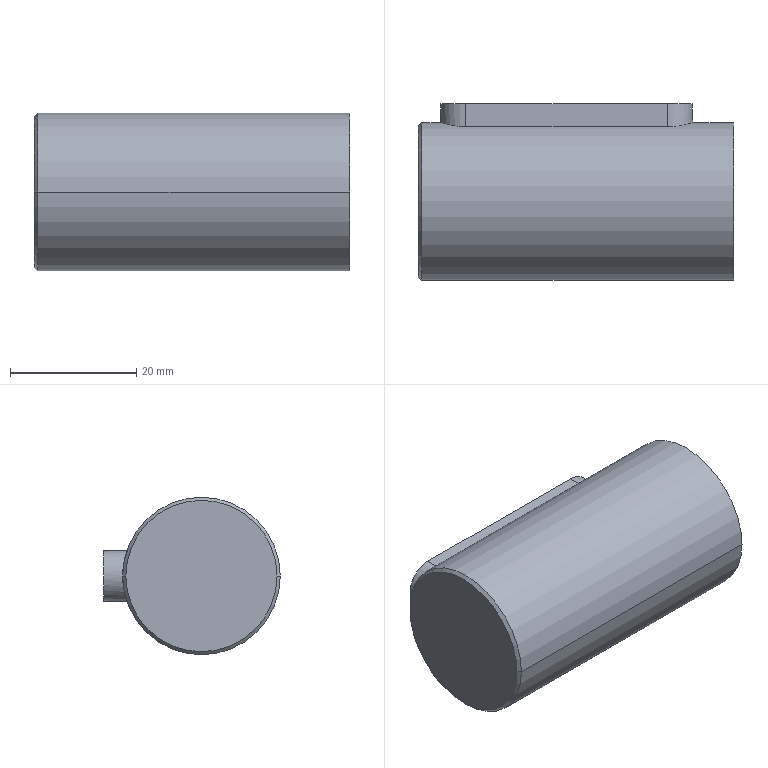Part | STEP file | PRODUCT_ID_83 | 1 solid | 11 faces | box 50 x 28 x 25 mm | volume 25516 mm3 | plane 5 | cylinder 4 | cone 2 | commonest cylinder face diameters 8 x2 25 x2
STEP:
#1=CARTESIAN_POINT('',(0.,0.,0.));
#2=DIRECTION('',(0.,0.,1.));
#3=DIRECTION('',(1.,0.,0.));
#4=AXIS2_PLACEMENT_3D('',#1,#2,#3);
#5=CARTESIAN_POINT('',(-42.5,15.5,4.));
#6=VERTEX_POINT('',#5);
#7=CARTESIAN_POINT('',(-42.5,15.5,-4.));
#8=VERTEX_POINT('',#7);
#9=CARTESIAN_POINT('',(-42.5,15.5,0.));
#10=DIRECTION('',(0.,-1.,0.));
#11=DIRECTION('',(0.,0.,1.));
#12=AXIS2_PLACEMENT_3D('',#9,#10,#11);
#13=CIRCLE('',#12,4.);
#14=CARTESIAN_POINT('',(-42.5,15.5,0.));
#15=DIRECTION('',(0.,1.,0.));
#16=DIRECTION('',(0.,0.,-1.));
#17=AXIS2_PLACEMENT_3D('',#14,#15,#16);
#18=PLANE('',#17);
#19=CARTESIAN_POINT('',(-4.,0.));
#20=CARTESIAN_POINT('',(-4.,6.928));
#21=CARTESIAN_POINT('',(2.,3.464));
#22=CARTESIAN_POINT('',(8.,0.));
#23=CARTESIAN_POINT('',(2.,-3.464));
#24=CARTESIAN_POINT('',(-4.,-6.928));
#25=CARTESIAN_POINT('',(-4.,0.));
#26=(BOUNDED_CURVE()B_SPLINE_CURVE(2,(#19,#20,#21,#22,#23,#24,#25),.UNSPECIFIED.,.T.,.F.)B_SPLINE_CURVE_WITH_KNOTS((1,2,2,2,2,1),(-2.094,0.,2.094,4.189,6.283,8.378),.UNSPECIFIED.)CURVE()GEOMETRIC_REPRESENTATION_ITEM()RATIONAL_B_SPLINE_CURVE((1.,0.5,1.,0.5,1.,0.5,1.))REPRESENTATION_ITEM(''));
#27=(GEOMETRIC_REPRESENTATION_CONTEXT(2)PARAMETRIC_REPRESENTATION_CONTEXT()REPRESENTATION_CONTEXT('',''));
#28=DEFINITIONAL_REPRESENTATION('',(#26),#27);
#29=PCURVE('',#18,#28);
#30=CARTESIAN_POINT('',(-42.5,7.75,0.));
#31=DIRECTION('',(0.,1.,0.));
#32=DIRECTION('',(0.,0.,1.));
#33=AXIS2_PLACEMENT_3D('',#30,#31,#32);
#34=CYLINDRICAL_SURFACE('',#33,4.);
#35=CARTESIAN_POINT('',(6.283,7.75));
#36=DIRECTION('',(-1.,0.));
#37=VECTOR('',#36,1.);
#38=LINE('',#35,#37);
#39=(GEOMETRIC_REPRESENTATION_CONTEXT(2)PARAMETRIC_REPRESENTATION_CONTEXT()REPRESENTATION_CONTEXT('',''));
#40=DEFINITIONAL_REPRESENTATION('',(#38),#39);
#41=PCURVE('',#34,#40);
#42=SURFACE_CURVE('',#13,(#29,#41),.PCURVE_S1.);
#43=EDGE_CURVE('',#6,#8,#42,.T.);
#44=ORIENTED_EDGE('',*,*,#43,.F.);
#45=CARTESIAN_POINT('',(-10.5,15.5,4.));
#46=VERTEX_POINT('',#45);
#47=CARTESIAN_POINT('',(-26.5,15.5,4.));
#48=DIRECTION('',(1.,0.,0.));
#49=VECTOR('',#48,1.);
#50=LINE('',#47,#49);
#51=CARTESIAN_POINT('',(-4.,-16.));
#52=DIRECTION('',(0.,-1.));
#53=VECTOR('',#52,1.);
#54=LINE('',#51,#53);
#55=(GEOMETRIC_REPRESENTATION_CONTEXT(2)PARAMETRIC_REPRESENTATION_CONTEXT()REPRESENTATION_CONTEXT('',''));
#56=DEFINITIONAL_REPRESENTATION('',(#54),#55);
#57=PCURVE('',#18,#56);
#58=CARTESIAN_POINT('',(-26.5,7.75,4.));
#59=DIRECTION('',(0.,0.,-1.));
#60=DIRECTION('',(0.,-1.,0.));
#61=AXIS2_PLACEMENT_3D('',#58,#59,#60);
#62=PLANE('',#61);
#63=CARTESIAN_POINT('',(-7.75,0.));
#64=DIRECTION('',(0.,-1.));
#65=VECTOR('',#64,1.);
#66=LINE('',#63,#65);
#67=(GEOMETRIC_REPRESENTATION_CONTEXT(2)PARAMETRIC_REPRESENTATION_CONTEXT()REPRESENTATION_CONTEXT('',''));
#68=DEFINITIONAL_REPRESENTATION('',(#66),#67);
#69=PCURVE('',#62,#68);
#70=SURFACE_CURVE('',#50,(#57,#69),.PCURVE_S1.);
#71=EDGE_CURVE('',#6,#46,#70,.T.);
#72=ORIENTED_EDGE('',*,*,#71,.T.);
#73=CARTESIAN_POINT('',(-10.5,15.5,-4.));
#74=VERTEX_POINT('',#73);
#75=CARTESIAN_POINT('',(-10.5,15.5,0.));
#76=DIRECTION('',(0.,-1.,0.));
#77=DIRECTION('',(0.,0.,1.));
#78=AXIS2_PLACEMENT_3D('',#75,#76,#77);
#79=CIRCLE('',#78,4.);
#80=CARTESIAN_POINT('',(-4.,-32.));
#81=CARTESIAN_POINT('',(-4.,-25.072));
#82=CARTESIAN_POINT('',(2.,-28.536));
#83=CARTESIAN_POINT('',(8.,-32.));
#84=CARTESIAN_POINT('',(2.,-35.464));
#85=CARTESIAN_POINT('',(-4.,-38.928));
#86=CARTESIAN_POINT('',(-4.,-32.));
#87=(BOUNDED_CURVE()B_SPLINE_CURVE(2,(#80,#81,#82,#83,#84,#85,#86),.UNSPECIFIED.,.T.,.F.)B_SPLINE_CURVE_WITH_KNOTS((1,2,2,2,2,1),(-2.094,0.,2.094,4.189,6.283,8.378),.UNSPECIFIED.)CURVE()GEOMETRIC_REPRESENTATION_ITEM()RATIONAL_B_SPLINE_CURVE((1.,0.5,1.,0.5,1.,0.5,1.))REPRESENTATION_ITEM(''));
#88=(GEOMETRIC_REPRESENTATION_CONTEXT(2)PARAMETRIC_REPRESENTATION_CONTEXT()REPRESENTATION_CONTEXT('',''));
#89=DEFINITIONAL_REPRESENTATION('',(#87),#88);
#90=PCURVE('',#18,#89);
#91=CARTESIAN_POINT('',(-10.5,7.75,0.));
#92=DIRECTION('',(0.,1.,0.));
#93=DIRECTION('',(0.,0.,1.));
#94=AXIS2_PLACEMENT_3D('',#91,#92,#93);
#95=CYLINDRICAL_SURFACE('',#94,4.);
#96=CARTESIAN_POINT('',(6.283,7.75));
#97=DIRECTION('',(-1.,0.));
#98=VECTOR('',#97,1.);
#99=LINE('',#96,#98);
#100=(GEOMETRIC_REPRESENTATION_CONTEXT(2)PARAMETRIC_REPRESENTATION_CONTEXT()REPRESENTATION_CONTEXT('',''));
#101=DEFINITIONAL_REPRESENTATION('',(#99),#100);
#102=PCURVE('',#95,#101);
#103=SURFACE_CURVE('',#79,(#90,#102),.PCURVE_S1.);
#104=EDGE_CURVE('',#74,#46,#103,.T.);
#105=ORIENTED_EDGE('',*,*,#104,.F.);
#106=CARTESIAN_POINT('',(-26.5,15.5,-4.));
#107=DIRECTION('',(-1.,0.,0.));
#108=VECTOR('',#107,1.);
#109=LINE('',#106,#108);
#110=CARTESIAN_POINT('',(4.,-16.));
#111=DIRECTION('',(0.,1.));
#112=VECTOR('',#111,1.);
#113=LINE('',#110,#112);
#114=(GEOMETRIC_REPRESENTATION_CONTEXT(2)PARAMETRIC_REPRESENTATION_CONTEXT()REPRESENTATION_CONTEXT('',''));
#115=DEFINITIONAL_REPRESENTATION('',(#113),#114);
#116=PCURVE('',#18,#115);
#117=CARTESIAN_POINT('',(-26.5,7.75,-4.));
#118=DIRECTION('',(0.,0.,1.));
#119=DIRECTION('',(0.,-1.,0.));
#120=AXIS2_PLACEMENT_3D('',#117,#118,#119);
#121=PLANE('',#120);
#122=CARTESIAN_POINT('',(-7.75,0.));
#123=DIRECTION('',(0.,-1.));
#124=VECTOR('',#123,1.);
#125=LINE('',#122,#124);
#126=(GEOMETRIC_REPRESENTATION_CONTEXT(2)PARAMETRIC_REPRESENTATION_CONTEXT()REPRESENTATION_CONTEXT('',''));
#127=DEFINITIONAL_REPRESENTATION('',(#125),#126);
#128=PCURVE('',#121,#127);
#129=SURFACE_CURVE('',#109,(#116,#128),.PCURVE_S1.);
#130=EDGE_CURVE('',#74,#8,#129,.T.);
#131=ORIENTED_EDGE('',*,*,#130,.T.);
#132=EDGE_LOOP('',(#44,#72,#105,#131));
#133=FACE_BOUND('',#132,.T.);
#134=ADVANCED_FACE('',(#133),#18,.T.);
#135=CARTESIAN_POINT('',(-50.,12.,0.));
#136=VERTEX_POINT('',#135);
#137=CARTESIAN_POINT('',(-50.,-12.,0.));
#138=VERTEX_POINT('',#137);
#139=CARTESIAN_POINT('',(-50.,0.,0.));
#140=DIRECTION('',(1.,0.,0.));
#141=DIRECTION('',(0.,1.,0.));
#142=AXIS2_PLACEMENT_3D('',#139,#140,#141);
#143=CIRCLE('',#142,12.);
#144=CARTESIAN_POINT('',(-50.,0.,0.));
#145=DIRECTION('',(1.,0.,0.));
#146=DIRECTION('',(0.,-1.,0.));
#147=AXIS2_PLACEMENT_3D('',#144,#145,#146);
#148=PLANE('',#147);
#149=CARTESIAN_POINT('',(0.,0.));
#150=DIRECTION('',(-1.,0.));
#151=AXIS2_PLACEMENT_2D('',#149,#150);
#152=CIRCLE('',#151,12.);
#153=(GEOMETRIC_REPRESENTATION_CONTEXT(2)PARAMETRIC_REPRESENTATION_CONTEXT()REPRESENTATION_CONTEXT('',''));
#154=DEFINITIONAL_REPRESENTATION('',(#152),#153);
#155=PCURVE('',#148,#154);
#156=CARTESIAN_POINT('',(-49.5,0.,0.));
#157=DIRECTION('',(1.,0.,0.));
#158=DIRECTION('',(0.,1.,0.));
#159=AXIS2_PLACEMENT_3D('',#156,#157,#158);
#160=CONICAL_SURFACE('',#159,12.5,0.7854);
#161=CARTESIAN_POINT('',(0.,-0.5));
#162=DIRECTION('',(1.,0.));
#163=VECTOR('',#162,1.);
#164=LINE('',#161,#163);
#165=(GEOMETRIC_REPRESENTATION_CONTEXT(2)PARAMETRIC_REPRESENTATION_CONTEXT()REPRESENTATION_CONTEXT('',''));
#166=DEFINITIONAL_REPRESENTATION('',(#164),#165);
#167=PCURVE('',#160,#166);
#168=SURFACE_CURVE('',#143,(#155,#167),.PCURVE_S1.);
#169=EDGE_CURVE('',#136,#138,#168,.T.);
#170=ORIENTED_EDGE('',*,*,#169,.F.);
#171=CARTESIAN_POINT('',(-50.,0.,0.));
#172=DIRECTION('',(1.,0.,0.));
#173=DIRECTION('',(0.,1.,0.));
#174=AXIS2_PLACEMENT_3D('',#171,#172,#173);
#175=CIRCLE('',#174,12.);
#176=CARTESIAN_POINT('',(0.,0.));
#177=DIRECTION('',(-1.,0.));
#178=AXIS2_PLACEMENT_2D('',#176,#177);
#179=CIRCLE('',#178,12.);
#180=(GEOMETRIC_REPRESENTATION_CONTEXT(2)PARAMETRIC_REPRESENTATION_CONTEXT()REPRESENTATION_CONTEXT('',''));
#181=DEFINITIONAL_REPRESENTATION('',(#179),#180);
#182=PCURVE('',#148,#181);
#183=CARTESIAN_POINT('',(-49.5,0.,0.));
#184=DIRECTION('',(1.,0.,0.));
#185=DIRECTION('',(0.,1.,0.));
#186=AXIS2_PLACEMENT_3D('',#183,#184,#185);
#187=CONICAL_SURFACE('',#186,12.5,0.7854);
#188=CARTESIAN_POINT('',(0.,-0.5));
#189=DIRECTION('',(1.,0.));
#190=VECTOR('',#189,1.);
#191=LINE('',#188,#190);
#192=(GEOMETRIC_REPRESENTATION_CONTEXT(2)PARAMETRIC_REPRESENTATION_CONTEXT()REPRESENTATION_CONTEXT('',''));
#193=DEFINITIONAL_REPRESENTATION('',(#191),#192);
#194=PCURVE('',#187,#193);
#195=SURFACE_CURVE('',#175,(#182,#194),.PCURVE_S1.);
#196=EDGE_CURVE('',#138,#136,#195,.T.);
#197=ORIENTED_EDGE('',*,*,#196,.F.);
#198=EDGE_LOOP('',(#170,#197));
#199=FACE_BOUND('',#198,.T.);
#200=ADVANCED_FACE('',(#199),#148,.F.);
#201=ORIENTED_EDGE('',*,*,#130,.F.);
#202=CARTESIAN_POINT('',(-10.5,11.843,-4.));
#203=VERTEX_POINT('',#202);
#204=CARTESIAN_POINT('',(-10.5,7.75,-4.));
#205=DIRECTION('',(0.,1.,0.));
#206=VECTOR('',#205,1.);
#207=LINE('',#204,#206);
#208=CARTESIAN_POINT('',(0.,16.));
#209=DIRECTION('',(-1.,0.));
#210=VECTOR('',#209,1.);
#211=LINE('',#208,#210);
#212=(GEOMETRIC_REPRESENTATION_CONTEXT(2)PARAMETRIC_REPRESENTATION_CONTEXT()REPRESENTATION_CONTEXT('',''));
#213=DEFINITIONAL_REPRESENTATION('',(#211),#212);
#214=PCURVE('',#121,#213);
#215=CARTESIAN_POINT('',(3.142,0.));
#216=DIRECTION('',(0.,1.));
#217=VECTOR('',#216,1.);
#218=LINE('',#215,#217);
#219=(GEOMETRIC_REPRESENTATION_CONTEXT(2)PARAMETRIC_REPRESENTATION_CONTEXT()REPRESENTATION_CONTEXT('',''));
#220=DEFINITIONAL_REPRESENTATION('',(#218),#219);
#221=PCURVE('',#95,#220);
#222=SURFACE_CURVE('',#207,(#214,#221),.PCURVE_S1.);
#223=EDGE_CURVE('',#203,#74,#222,.T.);
#224=ORIENTED_EDGE('',*,*,#223,.F.);
#225=CARTESIAN_POINT('',(-42.5,11.843,-4.));
#226=VERTEX_POINT('',#225);
#227=CARTESIAN_POINT('',(-24.75,11.843,-4.));
#228=DIRECTION('',(1.,0.,0.));
#229=VECTOR('',#228,1.);
#230=LINE('',#227,#229);
#231=CARTESIAN_POINT('',(-4.093,1.75));
#232=DIRECTION('',(0.,1.));
#233=VECTOR('',#232,1.);
#234=LINE('',#231,#233);
#235=(GEOMETRIC_REPRESENTATION_CONTEXT(2)PARAMETRIC_REPRESENTATION_CONTEXT()REPRESENTATION_CONTEXT('',''));
#236=DEFINITIONAL_REPRESENTATION('',(#234),#235);
#237=PCURVE('',#121,#236);
#238=CARTESIAN_POINT('',(-24.75,0.,0.));
#239=DIRECTION('',(-1.,0.,0.));
#240=DIRECTION('',(0.,-1.,0.));
#241=AXIS2_PLACEMENT_3D('',#238,#239,#240);
#242=CYLINDRICAL_SURFACE('',#241,12.5);
#243=CARTESIAN_POINT('',(3.467,0.));
#244=DIRECTION('',(0.,-1.));
#245=VECTOR('',#244,1.);
#246=LINE('',#243,#245);
#247=(GEOMETRIC_REPRESENTATION_CONTEXT(2)PARAMETRIC_REPRESENTATION_CONTEXT()REPRESENTATION_CONTEXT('',''));
#248=DEFINITIONAL_REPRESENTATION('',(#246),#247);
#249=PCURVE('',#242,#248);
#250=SURFACE_CURVE('',#230,(#237,#249),.PCURVE_S1.);
#251=EDGE_CURVE('',#226,#203,#250,.T.);
#252=ORIENTED_EDGE('',*,*,#251,.F.);
#253=CARTESIAN_POINT('',(-42.5,7.75,-4.));
#254=DIRECTION('',(0.,-1.,0.));
#255=VECTOR('',#254,1.);
#256=LINE('',#253,#255);
#257=CARTESIAN_POINT('',(0.,-16.));
#258=DIRECTION('',(1.,0.));
#259=VECTOR('',#258,1.);
#260=LINE('',#257,#259);
#261=(GEOMETRIC_REPRESENTATION_CONTEXT(2)PARAMETRIC_REPRESENTATION_CONTEXT()REPRESENTATION_CONTEXT('',''));
#262=DEFINITIONAL_REPRESENTATION('',(#260),#261);
#263=PCURVE('',#121,#262);
#264=CARTESIAN_POINT('',(3.142,0.));
#265=DIRECTION('',(0.,-1.));
#266=VECTOR('',#265,1.);
#267=LINE('',#264,#266);
#268=(GEOMETRIC_REPRESENTATION_CONTEXT(2)PARAMETRIC_REPRESENTATION_CONTEXT()REPRESENTATION_CONTEXT('',''));
#269=DEFINITIONAL_REPRESENTATION('',(#267),#268);
#270=PCURVE('',#34,#269);
#271=SURFACE_CURVE('',#256,(#263,#270),.PCURVE_S1.);
#272=EDGE_CURVE('',#8,#226,#271,.T.);
#273=ORIENTED_EDGE('',*,*,#272,.F.);
#274=EDGE_LOOP('',(#201,#224,#252,#273));
#275=FACE_BOUND('',#274,.T.);
#276=ADVANCED_FACE('',(#275),#121,.F.);
#277=CARTESIAN_POINT('',(0.,-12.5,0.));
#278=VERTEX_POINT('',#277);
#279=CARTESIAN_POINT('',(0.,12.5,0.));
#280=VERTEX_POINT('',#279);
#281=CARTESIAN_POINT('',(0.,0.,0.));
#282=DIRECTION('',(-1.,0.,0.));
#283=DIRECTION('',(0.,-1.,0.));
#284=AXIS2_PLACEMENT_3D('',#281,#282,#283);
#285=CIRCLE('',#284,12.5);
#286=CARTESIAN_POINT('',(0.,0.,0.));
#287=DIRECTION('',(1.,0.,0.));
#288=DIRECTION('',(0.,-1.,0.));
#289=AXIS2_PLACEMENT_3D('',#286,#287,#288);
#290=PLANE('',#289);
#291=CARTESIAN_POINT('',(12.5,0.));
#292=CARTESIAN_POINT('',(12.5,-21.651));
#293=CARTESIAN_POINT('',(-6.25,-10.825));
#294=CARTESIAN_POINT('',(-25.,0.));
#295=CARTESIAN_POINT('',(-6.25,10.825));
#296=CARTESIAN_POINT('',(12.5,21.651));
#297=CARTESIAN_POINT('',(12.5,0.));
#298=(BOUNDED_CURVE()B_SPLINE_CURVE(2,(#291,#292,#293,#294,#295,#296,#297),.UNSPECIFIED.,.T.,.F.)B_SPLINE_CURVE_WITH_KNOTS((1,2,2,2,2,1),(-2.094,0.,2.094,4.189,6.283,8.378),.UNSPECIFIED.)CURVE()GEOMETRIC_REPRESENTATION_ITEM()RATIONAL_B_SPLINE_CURVE((1.,0.5,1.,0.5,1.,0.5,1.))REPRESENTATION_ITEM(''));
#299=(GEOMETRIC_REPRESENTATION_CONTEXT(2)PARAMETRIC_REPRESENTATION_CONTEXT()REPRESENTATION_CONTEXT('',''));
#300=DEFINITIONAL_REPRESENTATION('',(#298),#299);
#301=PCURVE('',#290,#300);
#302=CARTESIAN_POINT('',(-24.75,0.,0.));
#303=DIRECTION('',(-1.,0.,0.));
#304=DIRECTION('',(0.,-1.,0.));
#305=AXIS2_PLACEMENT_3D('',#302,#303,#304);
#306=CYLINDRICAL_SURFACE('',#305,12.5);
#307=CARTESIAN_POINT('',(0.,-24.75));
#308=DIRECTION('',(1.,0.));
#309=VECTOR('',#308,1.);
#310=LINE('',#307,#309);
#311=(GEOMETRIC_REPRESENTATION_CONTEXT(2)PARAMETRIC_REPRESENTATION_CONTEXT()REPRESENTATION_CONTEXT('',''));
#312=DEFINITIONAL_REPRESENTATION('',(#310),#311);
#313=PCURVE('',#306,#312);
#314=SURFACE_CURVE('',#285,(#301,#313),.PCURVE_S1.);
#315=EDGE_CURVE('',#278,#280,#314,.T.);
#316=ORIENTED_EDGE('',*,*,#315,.F.);
#317=CARTESIAN_POINT('',(0.,0.,0.));
#318=DIRECTION('',(-1.,0.,0.));
#319=DIRECTION('',(0.,-1.,0.));
#320=AXIS2_PLACEMENT_3D('',#317,#318,#319);
#321=CIRCLE('',#320,12.5);
#322=CARTESIAN_POINT('',(12.5,0.));
#323=CARTESIAN_POINT('',(12.5,-21.651));
#324=CARTESIAN_POINT('',(-6.25,-10.825));
#325=CARTESIAN_POINT('',(-25.,0.));
#326=CARTESIAN_POINT('',(-6.25,10.825));
#327=CARTESIAN_POINT('',(12.5,21.651));
#328=CARTESIAN_POINT('',(12.5,0.));
#329=(BOUNDED_CURVE()B_SPLINE_CURVE(2,(#322,#323,#324,#325,#326,#327,#328),.UNSPECIFIED.,.T.,.F.)B_SPLINE_CURVE_WITH_KNOTS((1,2,2,2,2,1),(-2.094,0.,2.094,4.189,6.283,8.378),.UNSPECIFIED.)CURVE()GEOMETRIC_REPRESENTATION_ITEM()RATIONAL_B_SPLINE_CURVE((1.,0.5,1.,0.5,1.,0.5,1.))REPRESENTATION_ITEM(''));
#330=(GEOMETRIC_REPRESENTATION_CONTEXT(2)PARAMETRIC_REPRESENTATION_CONTEXT()REPRESENTATION_CONTEXT('',''));
#331=DEFINITIONAL_REPRESENTATION('',(#329),#330);
#332=PCURVE('',#290,#331);
#333=CARTESIAN_POINT('',(0.,-24.75));
#334=DIRECTION('',(1.,0.));
#335=VECTOR('',#334,1.);
#336=LINE('',#333,#335);
#337=(GEOMETRIC_REPRESENTATION_CONTEXT(2)PARAMETRIC_REPRESENTATION_CONTEXT()REPRESENTATION_CONTEXT('',''));
#338=DEFINITIONAL_REPRESENTATION('',(#336),#337);
#339=PCURVE('',#242,#338);
#340=SURFACE_CURVE('',#321,(#332,#339),.PCURVE_S1.);
#341=EDGE_CURVE('',#280,#278,#340,.T.);
#342=ORIENTED_EDGE('',*,*,#341,.F.);
#343=EDGE_LOOP('',(#316,#342));
#344=FACE_BOUND('',#343,.T.);
#345=ADVANCED_FACE('',(#344),#290,.T.);
#346=ORIENTED_EDGE('',*,*,#223,.T.);
#347=ORIENTED_EDGE('',*,*,#104,.T.);
#348=CARTESIAN_POINT('',(-10.5,11.843,4.));
#349=VERTEX_POINT('',#348);
#350=CARTESIAN_POINT('',(-10.5,7.75,4.));
#351=DIRECTION('',(0.,-1.,0.));
#352=VECTOR('',#351,1.);
#353=LINE('',#350,#352);
#354=CARTESIAN_POINT('',(0.,0.));
#355=DIRECTION('',(0.,-1.));
#356=VECTOR('',#355,1.);
#357=LINE('',#354,#356);
#358=(GEOMETRIC_REPRESENTATION_CONTEXT(2)PARAMETRIC_REPRESENTATION_CONTEXT()REPRESENTATION_CONTEXT('',''));
#359=DEFINITIONAL_REPRESENTATION('',(#357),#358);
#360=PCURVE('',#95,#359);
#361=CARTESIAN_POINT('',(0.,-16.));
#362=DIRECTION('',(1.,0.));
#363=VECTOR('',#362,1.);
#364=LINE('',#361,#363);
#365=(GEOMETRIC_REPRESENTATION_CONTEXT(2)PARAMETRIC_REPRESENTATION_CONTEXT()REPRESENTATION_CONTEXT('',''));
#366=DEFINITIONAL_REPRESENTATION('',(#364),#365);
#367=PCURVE('',#62,#366);
#368=SURFACE_CURVE('',#353,(#360,#367),.PCURVE_S1.);
#369=EDGE_CURVE('',#46,#349,#368,.T.);
#370=ORIENTED_EDGE('',*,*,#369,.T.);
#371=CARTESIAN_POINT('',(-6.5,12.5,0.));
#372=VERTEX_POINT('',#371);
#373=CARTESIAN_POINT('',(-6.5,12.5,0.));
#374=CARTESIAN_POINT('',(-6.5,12.5,0.2637));
#375=CARTESIAN_POINT('',(-6.526,12.492,0.5255));
#376=CARTESIAN_POINT('',(-6.603,12.467,0.9131));
#377=CARTESIAN_POINT('',(-6.635,12.457,1.041));
#378=CARTESIAN_POINT('',(-6.712,12.434,1.292));
#379=CARTESIAN_POINT('',(-6.757,12.42,1.417));
#380=CARTESIAN_POINT('',(-7.008,12.345,2.019));
#381=CARTESIAN_POINT('',(-7.302,12.262,2.459));
#382=CARTESIAN_POINT('',(-7.856,12.133,3.013));
#383=CARTESIAN_POINT('',(-8.055,12.091,3.176));
#384=CARTESIAN_POINT('',(-8.381,12.03,3.395));
#385=CARTESIAN_POINT('',(-8.493,12.011,3.463));
#386=CARTESIAN_POINT('',(-8.722,11.975,3.586));
#387=CARTESIAN_POINT('',(-8.838,11.958,3.641));
#388=CARTESIAN_POINT('',(-9.082,11.927,3.743));
#389=CARTESIAN_POINT('',(-9.206,11.913,3.787));
#390=CARTESIAN_POINT('',(-9.457,11.888,3.864));
#391=CARTESIAN_POINT('',(-9.583,11.877,3.896));
#392=CARTESIAN_POINT('',(-9.973,11.852,3.974));
#393=CARTESIAN_POINT('',(-10.235,11.843,4.));
#394=CARTESIAN_POINT('',(-10.5,11.843,4.));
#395=B_SPLINE_CURVE_WITH_KNOTS('',3,(#373,#374,#375,#376,#377,#378,#379,#380,#381,#382,#383,#384,#385,#386,#387,#388,#389,#390,#391,#392,#393,#394),.UNSPECIFIED.,.F.,.F.,(4,2,2,2,2,2,2,2,2,2,4),(0.,0.125,0.1875,0.25,0.5,0.625,0.6875,0.75,0.8125,0.875,1.),.UNSPECIFIED.);
#396=CARTESIAN_POINT('',(1.571,4.75));
#397=CARTESIAN_POINT('',(1.559,4.75));
#398=CARTESIAN_POINT('',(1.535,4.749));
#399=CARTESIAN_POINT('',(1.499,4.747));
#400=CARTESIAN_POINT('',(1.463,4.743));
#401=CARTESIAN_POINT('',(1.427,4.737));
#402=CARTESIAN_POINT('',(1.392,4.73));
#403=CARTESIAN_POINT('',(1.356,4.721));
#404=CARTESIAN_POINT('',(1.32,4.711));
#405=CARTESIAN_POINT('',(1.284,4.699));
#406=CARTESIAN_POINT('',(1.248,4.686));
#407=CARTESIAN_POINT('',(1.212,4.671));
#408=CARTESIAN_POINT('',(1.176,4.655));
#409=CARTESIAN_POINT('',(1.141,4.638));
#410=CARTESIAN_POINT('',(1.105,4.62));
#411=CARTESIAN_POINT('',(1.07,4.601));
#412=CARTESIAN_POINT('',(1.034,4.582));
#413=CARTESIAN_POINT('',(0.9987,4.561));
#414=CARTESIAN_POINT('',(0.9632,4.54));
#415=CARTESIAN_POINT('',(0.9277,4.518));
#416=CARTESIAN_POINT('',(0.8922,4.495));
#417=CARTESIAN_POINT('',(0.8567,4.472));
#418=CARTESIAN_POINT('',(0.8211,4.449));
#419=CARTESIAN_POINT('',(0.7855,4.426));
#420=CARTESIAN_POINT('',(0.7499,4.402));
#421=CARTESIAN_POINT('',(0.7146,4.379));
#422=CARTESIAN_POINT('',(0.6793,4.356));
#423=CARTESIAN_POINT('',(0.644,4.334));
#424=CARTESIAN_POINT('',(0.6085,4.311));
#425=CARTESIAN_POINT('',(0.5727,4.289));
#426=CARTESIAN_POINT('',(0.5371,4.268));
#427=CARTESIAN_POINT('',(0.5016,4.248));
#428=CARTESIAN_POINT('',(0.4662,4.228));
#429=CARTESIAN_POINT('',(0.4309,4.21));
#430=CARTESIAN_POINT('',(0.3952,4.192));
#431=CARTESIAN_POINT('',(0.3591,4.176));
#432=CARTESIAN_POINT('',(0.3233,4.16));
#433=CARTESIAN_POINT('',(0.2876,4.147));
#434=CARTESIAN_POINT('',(0.252,4.134));
#435=CARTESIAN_POINT('',(0.2163,4.124));
#436=CARTESIAN_POINT('',(0.1801,4.114));
#437=CARTESIAN_POINT('',(0.144,4.106));
#438=CARTESIAN_POINT('',(0.1081,4.1));
#439=CARTESIAN_POINT('',(0.07209,4.096));
#440=CARTESIAN_POINT('',(0.03609,4.093));
#441=CARTESIAN_POINT('',(0.01205,4.093));
#442=CARTESIAN_POINT('',(0.,4.093));
#443=B_SPLINE_CURVE_WITH_KNOTS('',3,(#396,#397,#398,#399,#400,#401,#402,#403,#404,#405,#406,#407,#408,#409,#410,#411,#412,#413,#414,#415,#416,#417,#418,#419,#420,#421,#422,#423,#424,#425,#426,#427,#428,#429,#430,#431,#432,#433,#434,#435,#436,#437,#438,#439,#440,#441,#442),.UNSPECIFIED.,.F.,.F.,(4,1,1,1,1,1,1,1,1,1,1,1,1,1,1,1,1,1,1,1,1,1,1,1,1,1,1,1,1,1,1,1,1,1,1,1,1,1,1,1,1,1,1,1,4),(0.,0.02273,0.04545,0.06818,0.09091,0.1136,0.1364,0.1591,0.1818,0.2045,0.2273,0.25,0.2727,0.2955,0.3182,0.3409,0.3636,0.3864,0.4091,0.4318,0.4545,0.4773,0.5,0.5227,0.5455,0.5682,0.5909,0.6136,0.6364,0.6591,0.6818,0.7045,0.7273,0.75,0.7727,0.7955,0.8182,0.8409,0.8636,0.8864,0.9091,0.9318,0.9545,0.9773,1.),.QUASI_UNIFORM_KNOTS.);
#444=(GEOMETRIC_REPRESENTATION_CONTEXT(2)PARAMETRIC_REPRESENTATION_CONTEXT()REPRESENTATION_CONTEXT('',''));
#445=DEFINITIONAL_REPRESENTATION('',(#443),#444);
#446=PCURVE('',#95,#445);
#447=CARTESIAN_POINT('',(3.142,-18.25));
#448=CARTESIAN_POINT('',(3.138,-18.25));
#449=CARTESIAN_POINT('',(3.13,-18.248));
#450=CARTESIAN_POINT('',(3.119,-18.241));
#451=CARTESIAN_POINT('',(3.107,-18.228));
#452=CARTESIAN_POINT('',(3.096,-18.21));
#453=CARTESIAN_POINT('',(3.084,-18.187));
#454=CARTESIAN_POINT('',(3.073,-18.159));
#455=CARTESIAN_POINT('',(3.062,-18.125));
#456=CARTESIAN_POINT('',(3.051,-18.087));
#457=CARTESIAN_POINT('',(3.04,-18.044));
#458=CARTESIAN_POINT('',(3.029,-17.996));
#459=CARTESIAN_POINT('',(3.018,-17.944));
#460=CARTESIAN_POINT('',(3.008,-17.887));
#461=CARTESIAN_POINT('',(2.997,-17.825));
#462=CARTESIAN_POINT('',(2.987,-17.759));
#463=CARTESIAN_POINT('',(2.977,-17.688));
#464=CARTESIAN_POINT('',(2.967,-17.614));
#465=CARTESIAN_POINT('',(2.958,-17.535));
#466=CARTESIAN_POINT('',(2.948,-17.452));
#467=CARTESIAN_POINT('',(2.939,-17.364));
#468=CARTESIAN_POINT('',(2.93,-17.273));
#469=CARTESIAN_POINT('',(2.922,-17.178));
#470=CARTESIAN_POINT('',(2.913,-17.079));
#471=CARTESIAN_POINT('',(2.905,-16.977));
#472=CARTESIAN_POINT('',(2.897,-16.872));
#473=CARTESIAN_POINT('',(2.89,-16.764));
#474=CARTESIAN_POINT('',(2.883,-16.652));
#475=CARTESIAN_POINT('',(2.876,-16.537));
#476=CARTESIAN_POINT('',(2.869,-16.418));
#477=CARTESIAN_POINT('',(2.863,-16.297));
#478=CARTESIAN_POINT('',(2.857,-16.174));
#479=CARTESIAN_POINT('',(2.852,-16.048));
#480=CARTESIAN_POINT('',(2.847,-15.921));
#481=CARTESIAN_POINT('',(2.842,-15.79));
#482=CARTESIAN_POINT('',(2.837,-15.656));
#483=CARTESIAN_POINT('',(2.833,-15.521));
#484=CARTESIAN_POINT('',(2.83,-15.385));
#485=CARTESIAN_POINT('',(2.826,-15.247));
#486=CARTESIAN_POINT('',(2.824,-15.108));
#487=CARTESIAN_POINT('',(2.821,-14.967));
#488=CARTESIAN_POINT('',(2.819,-14.824));
#489=CARTESIAN_POINT('',(2.818,-14.681));
#490=CARTESIAN_POINT('',(2.817,-14.538));
#491=CARTESIAN_POINT('',(2.816,-14.394));
#492=CARTESIAN_POINT('',(2.816,-14.298));
#493=CARTESIAN_POINT('',(2.816,-14.25));
#494=B_SPLINE_CURVE_WITH_KNOTS('',3,(#447,#448,#449,#450,#451,#452,#453,#454,#455,#456,#457,#458,#459,#460,#461,#462,#463,#464,#465,#466,#467,#468,#469,#470,#471,#472,#473,#474,#475,#476,#477,#478,#479,#480,#481,#482,#483,#484,#485,#486,#487,#488,#489,#490,#491,#492,#493),.UNSPECIFIED.,.F.,.F.,(4,1,1,1,1,1,1,1,1,1,1,1,1,1,1,1,1,1,1,1,1,1,1,1,1,1,1,1,1,1,1,1,1,1,1,1,1,1,1,1,1,1,1,1,4),(0.,0.02273,0.04545,0.06818,0.09091,0.1136,0.1364,0.1591,0.1818,0.2045,0.2273,0.25,0.2727,0.2955,0.3182,0.3409,0.3636,0.3864,0.4091,0.4318,0.4545,0.4773,0.5,0.5227,0.5455,0.5682,0.5909,0.6136,0.6364,0.6591,0.6818,0.7045,0.7273,0.75,0.7727,0.7955,0.8182,0.8409,0.8636,0.8864,0.9091,0.9318,0.9545,0.9773,1.),.QUASI_UNIFORM_KNOTS.);
#495=(GEOMETRIC_REPRESENTATION_CONTEXT(2)PARAMETRIC_REPRESENTATION_CONTEXT()REPRESENTATION_CONTEXT('',''));
#496=DEFINITIONAL_REPRESENTATION('',(#494),#495);
#497=PCURVE('',#306,#496);
#498=SURFACE_CURVE('',#395,(#446,#497),.PCURVE_S1.);
#499=EDGE_CURVE('',#372,#349,#498,.T.);
#500=ORIENTED_EDGE('',*,*,#499,.F.);
#501=CARTESIAN_POINT('',(-10.5,11.843,-4.));
#502=CARTESIAN_POINT('',(-10.236,11.843,-4.));
#503=CARTESIAN_POINT('',(-9.974,11.852,-3.974));
#504=CARTESIAN_POINT('',(-9.587,11.877,-3.897));
#505=CARTESIAN_POINT('',(-9.46,11.888,-3.865));
#506=CARTESIAN_POINT('',(-9.209,11.912,-3.788));
#507=CARTESIAN_POINT('',(-9.083,11.927,-3.743));
#508=CARTESIAN_POINT('',(-8.723,11.973,-3.593));
#509=CARTESIAN_POINT('',(-8.493,12.01,-3.47));
#510=CARTESIAN_POINT('',(-8.059,12.09,-3.18));
#511=CARTESIAN_POINT('',(-7.857,12.133,-3.013));
#512=CARTESIAN_POINT('',(-7.488,12.218,-2.645));
#513=CARTESIAN_POINT('',(-7.324,12.26,-2.445));
#514=CARTESIAN_POINT('',(-7.032,12.339,-2.011));
#515=CARTESIAN_POINT('',(-6.91,12.375,-1.783));
#516=CARTESIAN_POINT('',(-6.707,12.435,-1.297));
#517=CARTESIAN_POINT('',(-6.63,12.459,-1.047));
#518=CARTESIAN_POINT('',(-6.526,12.492,-0.5276));
#519=CARTESIAN_POINT('',(-6.5,12.5,-0.2649));
#520=CARTESIAN_POINT('',(-6.5,12.5,0.));
#521=B_SPLINE_CURVE_WITH_KNOTS('',3,(#501,#502,#503,#504,#505,#506,#507,#508,#509,#510,#511,#512,#513,#514,#515,#516,#517,#518,#519,#520),.UNSPECIFIED.,.F.,.F.,(4,2,2,2,2,2,2,2,2,4),(0.,0.125,0.1875,0.25,0.375,0.5,0.625,0.75,0.875,1.),.UNSPECIFIED.);
#522=CARTESIAN_POINT('',(3.142,4.093));
#523=CARTESIAN_POINT('',(3.13,4.093));
#524=CARTESIAN_POINT('',(3.106,4.093));
#525=CARTESIAN_POINT('',(3.07,4.096));
#526=CARTESIAN_POINT('',(3.034,4.1));
#527=CARTESIAN_POINT('',(2.998,4.106));
#528=CARTESIAN_POINT('',(2.962,4.114));
#529=CARTESIAN_POINT('',(2.926,4.123));
#530=CARTESIAN_POINT('',(2.891,4.134));
#531=CARTESIAN_POINT('',(2.855,4.146));
#532=CARTESIAN_POINT('',(2.819,4.16));
#533=CARTESIAN_POINT('',(2.783,4.175));
#534=CARTESIAN_POINT('',(2.747,4.192));
#535=CARTESIAN_POINT('',(2.712,4.209));
#536=CARTESIAN_POINT('',(2.676,4.228));
#537=CARTESIAN_POINT('',(2.641,4.247));
#538=CARTESIAN_POINT('',(2.605,4.268));
#539=CARTESIAN_POINT('',(2.57,4.289));
#540=CARTESIAN_POINT('',(2.534,4.311));
#541=CARTESIAN_POINT('',(2.499,4.333));
#542=CARTESIAN_POINT('',(2.463,4.356));
#543=CARTESIAN_POINT('',(2.428,4.379));
#544=CARTESIAN_POINT('',(2.392,4.402));
#545=CARTESIAN_POINT('',(2.357,4.426));
#546=CARTESIAN_POINT('',(2.321,4.449));
#547=CARTESIAN_POINT('',(2.286,4.472));
#548=CARTESIAN_POINT('',(2.25,4.495));
#549=CARTESIAN_POINT('',(2.215,4.517));
#550=CARTESIAN_POINT('',(2.179,4.539));
#551=CARTESIAN_POINT('',(2.144,4.561));
#552=CARTESIAN_POINT('',(2.108,4.581));
#553=CARTESIAN_POINT('',(2.073,4.601));
#554=CARTESIAN_POINT('',(2.037,4.62));
#555=CARTESIAN_POINT('',(2.002,4.638));
#556=CARTESIAN_POINT('',(1.966,4.655));
#557=CARTESIAN_POINT('',(1.93,4.671));
#558=CARTESIAN_POINT('',(1.894,4.685));
#559=CARTESIAN_POINT('',(1.859,4.699));
#560=CARTESIAN_POINT('',(1.823,4.71));
#561=CARTESIAN_POINT('',(1.787,4.721));
#562=CARTESIAN_POINT('',(1.751,4.73));
#563=CARTESIAN_POINT('',(1.715,4.737));
#564=CARTESIAN_POINT('',(1.679,4.743));
#565=CARTESIAN_POINT('',(1.643,4.747));
#566=CARTESIAN_POINT('',(1.607,4.749));
#567=CARTESIAN_POINT('',(1.583,4.75));
#568=CARTESIAN_POINT('',(1.571,4.75));
#569=B_SPLINE_CURVE_WITH_KNOTS('',3,(#522,#523,#524,#525,#526,#527,#528,#529,#530,#531,#532,#533,#534,#535,#536,#537,#538,#539,#540,#541,#542,#543,#544,#545,#546,#547,#548,#549,#550,#551,#552,#553,#554,#555,#556,#557,#558,#559,#560,#561,#562,#563,#564,#565,#566,#567,#568),.UNSPECIFIED.,.F.,.F.,(4,1,1,1,1,1,1,1,1,1,1,1,1,1,1,1,1,1,1,1,1,1,1,1,1,1,1,1,1,1,1,1,1,1,1,1,1,1,1,1,1,1,1,1,4),(0.,0.02273,0.04545,0.06818,0.09091,0.1136,0.1364,0.1591,0.1818,0.2045,0.2273,0.25,0.2727,0.2955,0.3182,0.3409,0.3636,0.3864,0.4091,0.4318,0.4545,0.4773,0.5,0.5227,0.5455,0.5682,0.5909,0.6136,0.6364,0.6591,0.6818,0.7045,0.7273,0.75,0.7727,0.7955,0.8182,0.8409,0.8636,0.8864,0.9091,0.9318,0.9545,0.9773,1.),.QUASI_UNIFORM_KNOTS.);
#570=(GEOMETRIC_REPRESENTATION_CONTEXT(2)PARAMETRIC_REPRESENTATION_CONTEXT()REPRESENTATION_CONTEXT('',''));
#571=DEFINITIONAL_REPRESENTATION('',(#569),#570);
#572=PCURVE('',#95,#571);
#573=CARTESIAN_POINT('',(3.467,-14.25));
#574=CARTESIAN_POINT('',(3.467,-14.298));
#575=CARTESIAN_POINT('',(3.467,-14.394));
#576=CARTESIAN_POINT('',(3.467,-14.537));
#577=CARTESIAN_POINT('',(3.465,-14.68));
#578=CARTESIAN_POINT('',(3.464,-14.822));
#579=CARTESIAN_POINT('',(3.462,-14.964));
#580=CARTESIAN_POINT('',(3.46,-15.104));
#581=CARTESIAN_POINT('',(3.457,-15.244));
#582=CARTESIAN_POINT('',(3.454,-15.381));
#583=CARTESIAN_POINT('',(3.45,-15.518));
#584=CARTESIAN_POINT('',(3.446,-15.654));
#585=CARTESIAN_POINT('',(3.442,-15.787));
#586=CARTESIAN_POINT('',(3.437,-15.917));
#587=CARTESIAN_POINT('',(3.432,-16.045));
#588=CARTESIAN_POINT('',(3.426,-16.171));
#589=CARTESIAN_POINT('',(3.42,-16.294));
#590=CARTESIAN_POINT('',(3.414,-16.415));
#591=CARTESIAN_POINT('',(3.408,-16.533));
#592=CARTESIAN_POINT('',(3.401,-16.649));
#593=CARTESIAN_POINT('',(3.393,-16.761));
#594=CARTESIAN_POINT('',(3.386,-16.87));
#595=CARTESIAN_POINT('',(3.378,-16.976));
#596=CARTESIAN_POINT('',(3.37,-17.078));
#597=CARTESIAN_POINT('',(3.362,-17.177));
#598=CARTESIAN_POINT('',(3.353,-17.271));
#599=CARTESIAN_POINT('',(3.344,-17.362));
#600=CARTESIAN_POINT('',(3.335,-17.449));
#601=CARTESIAN_POINT('',(3.326,-17.532));
#602=CARTESIAN_POINT('',(3.316,-17.612));
#603=CARTESIAN_POINT('',(3.306,-17.687));
#604=CARTESIAN_POINT('',(3.296,-17.757));
#605=CARTESIAN_POINT('',(3.286,-17.823));
#606=CARTESIAN_POINT('',(3.276,-17.885));
#607=CARTESIAN_POINT('',(3.265,-17.942));
#608=CARTESIAN_POINT('',(3.254,-17.995));
#609=CARTESIAN_POINT('',(3.244,-18.043));
#610=CARTESIAN_POINT('',(3.233,-18.086));
#611=CARTESIAN_POINT('',(3.222,-18.124));
#612=CARTESIAN_POINT('',(3.21,-18.158));
#613=CARTESIAN_POINT('',(3.199,-18.186));
#614=CARTESIAN_POINT('',(3.188,-18.209));
#615=CARTESIAN_POINT('',(3.176,-18.228));
#616=CARTESIAN_POINT('',(3.165,-18.241));
#617=CARTESIAN_POINT('',(3.153,-18.248));
#618=CARTESIAN_POINT('',(3.145,-18.25));
#619=CARTESIAN_POINT('',(3.142,-18.25));
#620=B_SPLINE_CURVE_WITH_KNOTS('',3,(#573,#574,#575,#576,#577,#578,#579,#580,#581,#582,#583,#584,#585,#586,#587,#588,#589,#590,#591,#592,#593,#594,#595,#596,#597,#598,#599,#600,#601,#602,#603,#604,#605,#606,#607,#608,#609,#610,#611,#612,#613,#614,#615,#616,#617,#618,#619),.UNSPECIFIED.,.F.,.F.,(4,1,1,1,1,1,1,1,1,1,1,1,1,1,1,1,1,1,1,1,1,1,1,1,1,1,1,1,1,1,1,1,1,1,1,1,1,1,1,1,1,1,1,1,4),(0.,0.02273,0.04545,0.06818,0.09091,0.1136,0.1364,0.1591,0.1818,0.2045,0.2273,0.25,0.2727,0.2955,0.3182,0.3409,0.3636,0.3864,0.4091,0.4318,0.4545,0.4773,0.5,0.5227,0.5455,0.5682,0.5909,0.6136,0.6364,0.6591,0.6818,0.7045,0.7273,0.75,0.7727,0.7955,0.8182,0.8409,0.8636,0.8864,0.9091,0.9318,0.9545,0.9773,1.),.QUASI_UNIFORM_KNOTS.);
#621=(GEOMETRIC_REPRESENTATION_CONTEXT(2)PARAMETRIC_REPRESENTATION_CONTEXT()REPRESENTATION_CONTEXT('',''));
#622=DEFINITIONAL_REPRESENTATION('',(#620),#621);
#623=PCURVE('',#242,#622);
#624=SURFACE_CURVE('',#521,(#572,#623),.PCURVE_S1.);
#625=EDGE_CURVE('',#203,#372,#624,.T.);
#626=ORIENTED_EDGE('',*,*,#625,.F.);
#627=EDGE_LOOP('',(#346,#347,#370,#500,#626));
#628=FACE_BOUND('',#627,.T.);
#629=ADVANCED_FACE('',(#628),#95,.T.);
#630=ORIENTED_EDGE('',*,*,#71,.F.);
#631=CARTESIAN_POINT('',(-42.5,11.843,4.));
#632=VERTEX_POINT('',#631);
#633=CARTESIAN_POINT('',(-42.5,7.75,4.));
#634=DIRECTION('',(0.,1.,0.));
#635=VECTOR('',#634,1.);
#636=LINE('',#633,#635);
#637=CARTESIAN_POINT('',(0.,16.));
#638=DIRECTION('',(-1.,0.));
#639=VECTOR('',#638,1.);
#640=LINE('',#637,#639);
#641=(GEOMETRIC_REPRESENTATION_CONTEXT(2)PARAMETRIC_REPRESENTATION_CONTEXT()REPRESENTATION_CONTEXT('',''));
#642=DEFINITIONAL_REPRESENTATION('',(#640),#641);
#643=PCURVE('',#62,#642);
#644=CARTESIAN_POINT('',(6.283,0.));
#645=DIRECTION('',(0.,1.));
#646=VECTOR('',#645,1.);
#647=LINE('',#644,#646);
#648=(GEOMETRIC_REPRESENTATION_CONTEXT(2)PARAMETRIC_REPRESENTATION_CONTEXT()REPRESENTATION_CONTEXT('',''));
#649=DEFINITIONAL_REPRESENTATION('',(#647),#648);
#650=PCURVE('',#34,#649);
#651=SURFACE_CURVE('',#636,(#643,#650),.PCURVE_S1.);
#652=EDGE_CURVE('',#632,#6,#651,.T.);
#653=ORIENTED_EDGE('',*,*,#652,.F.);
#654=CARTESIAN_POINT('',(-24.75,11.843,4.));
#655=DIRECTION('',(-1.,0.,0.));
#656=VECTOR('',#655,1.);
#657=LINE('',#654,#656);
#658=CARTESIAN_POINT('',(-4.093,-1.75));
#659=DIRECTION('',(0.,1.));
#660=VECTOR('',#659,1.);
#661=LINE('',#658,#660);
#662=(GEOMETRIC_REPRESENTATION_CONTEXT(2)PARAMETRIC_REPRESENTATION_CONTEXT()REPRESENTATION_CONTEXT('',''));
#663=DEFINITIONAL_REPRESENTATION('',(#661),#662);
#664=PCURVE('',#62,#663);
#665=CARTESIAN_POINT('',(2.816,0.));
#666=DIRECTION('',(0.,1.));
#667=VECTOR('',#666,1.);
#668=LINE('',#665,#667);
#669=(GEOMETRIC_REPRESENTATION_CONTEXT(2)PARAMETRIC_REPRESENTATION_CONTEXT()REPRESENTATION_CONTEXT('',''));
#670=DEFINITIONAL_REPRESENTATION('',(#668),#669);
#671=PCURVE('',#306,#670);
#672=SURFACE_CURVE('',#657,(#664,#671),.PCURVE_S1.);
#673=EDGE_CURVE('',#349,#632,#672,.T.);
#674=ORIENTED_EDGE('',*,*,#673,.F.);
#675=ORIENTED_EDGE('',*,*,#369,.F.);
#676=EDGE_LOOP('',(#630,#653,#674,#675));
#677=FACE_BOUND('',#676,.T.);
#678=ADVANCED_FACE('',(#677),#62,.F.);
#679=ORIENTED_EDGE('',*,*,#272,.T.);
#680=CARTESIAN_POINT('',(-46.5,12.5,0.));
#681=VERTEX_POINT('',#680);
#682=CARTESIAN_POINT('',(-46.5,12.5,0.));
#683=CARTESIAN_POINT('',(-46.5,12.5,-0.2637));
#684=CARTESIAN_POINT('',(-46.474,12.492,-0.5255));
#685=CARTESIAN_POINT('',(-46.397,12.467,-0.9131));
#686=CARTESIAN_POINT('',(-46.365,12.457,-1.041));
#687=CARTESIAN_POINT('',(-46.288,12.434,-1.292));
#688=CARTESIAN_POINT('',(-46.243,12.42,-1.417));
#689=CARTESIAN_POINT('',(-45.992,12.345,-2.019));
#690=CARTESIAN_POINT('',(-45.698,12.262,-2.459));
#691=CARTESIAN_POINT('',(-45.144,12.133,-3.013));
#692=CARTESIAN_POINT('',(-44.945,12.091,-3.176));
#693=CARTESIAN_POINT('',(-44.619,12.03,-3.395));
#694=CARTESIAN_POINT('',(-44.507,12.011,-3.463));
#695=CARTESIAN_POINT('',(-44.278,11.975,-3.586));
#696=CARTESIAN_POINT('',(-44.162,11.958,-3.641));
#697=CARTESIAN_POINT('',(-43.918,11.927,-3.743));
#698=CARTESIAN_POINT('',(-43.794,11.913,-3.787));
#699=CARTESIAN_POINT('',(-43.543,11.888,-3.864));
#700=CARTESIAN_POINT('',(-43.417,11.877,-3.896));
#701=CARTESIAN_POINT('',(-43.027,11.852,-3.974));
#702=CARTESIAN_POINT('',(-42.765,11.843,-4.));
#703=CARTESIAN_POINT('',(-42.5,11.843,-4.));
#704=B_SPLINE_CURVE_WITH_KNOTS('',3,(#682,#683,#684,#685,#686,#687,#688,#689,#690,#691,#692,#693,#694,#695,#696,#697,#698,#699,#700,#701,#702,#703),.UNSPECIFIED.,.F.,.F.,(4,2,2,2,2,2,2,2,2,2,4),(0.,0.125,0.1875,0.25,0.5,0.625,0.6875,0.75,0.8125,0.875,1.),.UNSPECIFIED.);
#705=CARTESIAN_POINT('',(4.712,4.75));
#706=CARTESIAN_POINT('',(4.7,4.75));
#707=CARTESIAN_POINT('',(4.676,4.749));
#708=CARTESIAN_POINT('',(4.641,4.747));
#709=CARTESIAN_POINT('',(4.605,4.743));
#710=CARTESIAN_POINT('',(4.569,4.737));
#711=CARTESIAN_POINT('',(4.533,4.73));
#712=CARTESIAN_POINT('',(4.497,4.721));
#713=CARTESIAN_POINT('',(4.461,4.711));
#714=CARTESIAN_POINT('',(4.426,4.699));
#715=CARTESIAN_POINT('',(4.39,4.686));
#716=CARTESIAN_POINT('',(4.354,4.671));
#717=CARTESIAN_POINT('',(4.318,4.655));
#718=CARTESIAN_POINT('',(4.282,4.638));
#719=CARTESIAN_POINT('',(4.247,4.62));
#720=CARTESIAN_POINT('',(4.211,4.601));
#721=CARTESIAN_POINT('',(4.176,4.582));
#722=CARTESIAN_POINT('',(4.14,4.561));
#723=CARTESIAN_POINT('',(4.105,4.54));
#724=CARTESIAN_POINT('',(4.069,4.518));
#725=CARTESIAN_POINT('',(4.034,4.495));
#726=CARTESIAN_POINT('',(3.998,4.472));
#727=CARTESIAN_POINT('',(3.963,4.449));
#728=CARTESIAN_POINT('',(3.927,4.426));
#729=CARTESIAN_POINT('',(3.892,4.402));
#730=CARTESIAN_POINT('',(3.856,4.379));
#731=CARTESIAN_POINT('',(3.821,4.356));
#732=CARTESIAN_POINT('',(3.786,4.334));
#733=CARTESIAN_POINT('',(3.75,4.311));
#734=CARTESIAN_POINT('',(3.714,4.289));
#735=CARTESIAN_POINT('',(3.679,4.268));
#736=CARTESIAN_POINT('',(3.643,4.248));
#737=CARTESIAN_POINT('',(3.608,4.228));
#738=CARTESIAN_POINT('',(3.573,4.21));
#739=CARTESIAN_POINT('',(3.537,4.192));
#740=CARTESIAN_POINT('',(3.501,4.176));
#741=CARTESIAN_POINT('',(3.465,4.16));
#742=CARTESIAN_POINT('',(3.429,4.147));
#743=CARTESIAN_POINT('',(3.394,4.134));
#744=CARTESIAN_POINT('',(3.358,4.124));
#745=CARTESIAN_POINT('',(3.322,4.114));
#746=CARTESIAN_POINT('',(3.286,4.106));
#747=CARTESIAN_POINT('',(3.25,4.1));
#748=CARTESIAN_POINT('',(3.214,4.096));
#749=CARTESIAN_POINT('',(3.178,4.093));
#750=CARTESIAN_POINT('',(3.154,4.093));
#751=CARTESIAN_POINT('',(3.142,4.093));
#752=B_SPLINE_CURVE_WITH_KNOTS('',3,(#705,#706,#707,#708,#709,#710,#711,#712,#713,#714,#715,#716,#717,#718,#719,#720,#721,#722,#723,#724,#725,#726,#727,#728,#729,#730,#731,#732,#733,#734,#735,#736,#737,#738,#739,#740,#741,#742,#743,#744,#745,#746,#747,#748,#749,#750,#751),.UNSPECIFIED.,.F.,.F.,(4,1,1,1,1,1,1,1,1,1,1,1,1,1,1,1,1,1,1,1,1,1,1,1,1,1,1,1,1,1,1,1,1,1,1,1,1,1,1,1,1,1,1,1,4),(0.,0.02273,0.04545,0.06818,0.09091,0.1136,0.1364,0.1591,0.1818,0.2045,0.2273,0.25,0.2727,0.2955,0.3182,0.3409,0.3636,0.3864,0.4091,0.4318,0.4545,0.4773,0.5,0.5227,0.5455,0.5682,0.5909,0.6136,0.6364,0.6591,0.6818,0.7045,0.7273,0.75,0.7727,0.7955,0.8182,0.8409,0.8636,0.8864,0.9091,0.9318,0.9545,0.9773,1.),.QUASI_UNIFORM_KNOTS.);
#753=(GEOMETRIC_REPRESENTATION_CONTEXT(2)PARAMETRIC_REPRESENTATION_CONTEXT()REPRESENTATION_CONTEXT('',''));
#754=DEFINITIONAL_REPRESENTATION('',(#752),#753);
#755=PCURVE('',#34,#754);
#756=CARTESIAN_POINT('',(3.142,21.75));
#757=CARTESIAN_POINT('',(3.145,21.75));
#758=CARTESIAN_POINT('',(3.153,21.748));
#759=CARTESIAN_POINT('',(3.165,21.741));
#760=CARTESIAN_POINT('',(3.176,21.728));
#761=CARTESIAN_POINT('',(3.187,21.71));
#762=CARTESIAN_POINT('',(3.199,21.687));
#763=CARTESIAN_POINT('',(3.21,21.659));
#764=CARTESIAN_POINT('',(3.221,21.625));
#765=CARTESIAN_POINT('',(3.232,21.587));
#766=CARTESIAN_POINT('',(3.243,21.544));
#767=CARTESIAN_POINT('',(3.254,21.496));
#768=CARTESIAN_POINT('',(3.265,21.444));
#769=CARTESIAN_POINT('',(3.275,21.387));
#770=CARTESIAN_POINT('',(3.286,21.325));
#771=CARTESIAN_POINT('',(3.296,21.259));
#772=CARTESIAN_POINT('',(3.306,21.188));
#773=CARTESIAN_POINT('',(3.316,21.114));
#774=CARTESIAN_POINT('',(3.325,21.035));
#775=CARTESIAN_POINT('',(3.335,20.952));
#776=CARTESIAN_POINT('',(3.344,20.864));
#777=CARTESIAN_POINT('',(3.353,20.773));
#778=CARTESIAN_POINT('',(3.361,20.678));
#779=CARTESIAN_POINT('',(3.37,20.579));
#780=CARTESIAN_POINT('',(3.378,20.477));
#781=CARTESIAN_POINT('',(3.386,20.372));
#782=CARTESIAN_POINT('',(3.393,20.264));
#783=CARTESIAN_POINT('',(3.4,20.152));
#784=CARTESIAN_POINT('',(3.407,20.037));
#785=CARTESIAN_POINT('',(3.414,19.918));
#786=CARTESIAN_POINT('',(3.42,19.797));
#787=CARTESIAN_POINT('',(3.426,19.674));
#788=CARTESIAN_POINT('',(3.432,19.548));
#789=CARTESIAN_POINT('',(3.437,19.421));
#790=CARTESIAN_POINT('',(3.441,19.29));
#791=CARTESIAN_POINT('',(3.446,19.156));
#792=CARTESIAN_POINT('',(3.45,19.021));
#793=CARTESIAN_POINT('',(3.454,18.885));
#794=CARTESIAN_POINT('',(3.457,18.747));
#795=CARTESIAN_POINT('',(3.46,18.608));
#796=CARTESIAN_POINT('',(3.462,18.467));
#797=CARTESIAN_POINT('',(3.464,18.324));
#798=CARTESIAN_POINT('',(3.465,18.181));
#799=CARTESIAN_POINT('',(3.467,18.038));
#800=CARTESIAN_POINT('',(3.467,17.894));
#801=CARTESIAN_POINT('',(3.467,17.798));
#802=CARTESIAN_POINT('',(3.467,17.75));
#803=B_SPLINE_CURVE_WITH_KNOTS('',3,(#756,#757,#758,#759,#760,#761,#762,#763,#764,#765,#766,#767,#768,#769,#770,#771,#772,#773,#774,#775,#776,#777,#778,#779,#780,#781,#782,#783,#784,#785,#786,#787,#788,#789,#790,#791,#792,#793,#794,#795,#796,#797,#798,#799,#800,#801,#802),.UNSPECIFIED.,.F.,.F.,(4,1,1,1,1,1,1,1,1,1,1,1,1,1,1,1,1,1,1,1,1,1,1,1,1,1,1,1,1,1,1,1,1,1,1,1,1,1,1,1,1,1,1,1,4),(0.,0.02273,0.04545,0.06818,0.09091,0.1136,0.1364,0.1591,0.1818,0.2045,0.2273,0.25,0.2727,0.2955,0.3182,0.3409,0.3636,0.3864,0.4091,0.4318,0.4545,0.4773,0.5,0.5227,0.5455,0.5682,0.5909,0.6136,0.6364,0.6591,0.6818,0.7045,0.7273,0.75,0.7727,0.7955,0.8182,0.8409,0.8636,0.8864,0.9091,0.9318,0.9545,0.9773,1.),.QUASI_UNIFORM_KNOTS.);
#804=(GEOMETRIC_REPRESENTATION_CONTEXT(2)PARAMETRIC_REPRESENTATION_CONTEXT()REPRESENTATION_CONTEXT('',''));
#805=DEFINITIONAL_REPRESENTATION('',(#803),#804);
#806=PCURVE('',#242,#805);
#807=SURFACE_CURVE('',#704,(#755,#806),.PCURVE_S1.);
#808=EDGE_CURVE('',#681,#226,#807,.T.);
#809=ORIENTED_EDGE('',*,*,#808,.F.);
#810=CARTESIAN_POINT('',(-42.5,11.843,4.));
#811=CARTESIAN_POINT('',(-42.764,11.843,4.));
#812=CARTESIAN_POINT('',(-43.026,11.852,3.974));
#813=CARTESIAN_POINT('',(-43.413,11.877,3.897));
#814=CARTESIAN_POINT('',(-43.54,11.888,3.865));
#815=CARTESIAN_POINT('',(-43.791,11.912,3.788));
#816=CARTESIAN_POINT('',(-43.917,11.927,3.743));
#817=CARTESIAN_POINT('',(-44.277,11.973,3.593));
#818=CARTESIAN_POINT('',(-44.507,12.01,3.47));
#819=CARTESIAN_POINT('',(-44.941,12.09,3.18));
#820=CARTESIAN_POINT('',(-45.143,12.133,3.013));
#821=CARTESIAN_POINT('',(-45.512,12.218,2.645));
#822=CARTESIAN_POINT('',(-45.676,12.26,2.445));
#823=CARTESIAN_POINT('',(-45.968,12.339,2.011));
#824=CARTESIAN_POINT('',(-46.09,12.375,1.783));
#825=CARTESIAN_POINT('',(-46.293,12.435,1.297));
#826=CARTESIAN_POINT('',(-46.37,12.459,1.047));
#827=CARTESIAN_POINT('',(-46.474,12.492,0.5276));
#828=CARTESIAN_POINT('',(-46.5,12.5,0.2649));
#829=CARTESIAN_POINT('',(-46.5,12.5,0.));
#830=B_SPLINE_CURVE_WITH_KNOTS('',3,(#810,#811,#812,#813,#814,#815,#816,#817,#818,#819,#820,#821,#822,#823,#824,#825,#826,#827,#828,#829),.UNSPECIFIED.,.F.,.F.,(4,2,2,2,2,2,2,2,2,4),(0.,0.125,0.1875,0.25,0.375,0.5,0.625,0.75,0.875,1.),.UNSPECIFIED.);
#831=CARTESIAN_POINT('',(6.283,4.093));
#832=CARTESIAN_POINT('',(6.271,4.093));
#833=CARTESIAN_POINT('',(6.247,4.093));
#834=CARTESIAN_POINT('',(6.211,4.096));
#835=CARTESIAN_POINT('',(6.176,4.1));
#836=CARTESIAN_POINT('',(6.14,4.106));
#837=CARTESIAN_POINT('',(6.104,4.114));
#838=CARTESIAN_POINT('',(6.068,4.123));
#839=CARTESIAN_POINT('',(6.032,4.134));
#840=CARTESIAN_POINT('',(5.996,4.146));
#841=CARTESIAN_POINT('',(5.961,4.16));
#842=CARTESIAN_POINT('',(5.925,4.175));
#843=CARTESIAN_POINT('',(5.889,4.192));
#844=CARTESIAN_POINT('',(5.853,4.209));
#845=CARTESIAN_POINT('',(5.818,4.228));
#846=CARTESIAN_POINT('',(5.782,4.247));
#847=CARTESIAN_POINT('',(5.747,4.268));
#848=CARTESIAN_POINT('',(5.711,4.289));
#849=CARTESIAN_POINT('',(5.676,4.311));
#850=CARTESIAN_POINT('',(5.64,4.333));
#851=CARTESIAN_POINT('',(5.605,4.356));
#852=CARTESIAN_POINT('',(5.569,4.379));
#853=CARTESIAN_POINT('',(5.534,4.402));
#854=CARTESIAN_POINT('',(5.498,4.426));
#855=CARTESIAN_POINT('',(5.463,4.449));
#856=CARTESIAN_POINT('',(5.427,4.472));
#857=CARTESIAN_POINT('',(5.392,4.495));
#858=CARTESIAN_POINT('',(5.357,4.517));
#859=CARTESIAN_POINT('',(5.321,4.539));
#860=CARTESIAN_POINT('',(5.285,4.561));
#861=CARTESIAN_POINT('',(5.25,4.581));
#862=CARTESIAN_POINT('',(5.214,4.601));
#863=CARTESIAN_POINT('',(5.179,4.62));
#864=CARTESIAN_POINT('',(5.143,4.638));
#865=CARTESIAN_POINT('',(5.108,4.655));
#866=CARTESIAN_POINT('',(5.072,4.671));
#867=CARTESIAN_POINT('',(5.036,4.685));
#868=CARTESIAN_POINT('',(5.,4.699));
#869=CARTESIAN_POINT('',(4.965,4.71));
#870=CARTESIAN_POINT('',(4.929,4.721));
#871=CARTESIAN_POINT('',(4.892,4.73));
#872=CARTESIAN_POINT('',(4.856,4.737));
#873=CARTESIAN_POINT('',(4.82,4.743));
#874=CARTESIAN_POINT('',(4.784,4.747));
#875=CARTESIAN_POINT('',(4.748,4.749));
#876=CARTESIAN_POINT('',(4.724,4.75));
#877=CARTESIAN_POINT('',(4.712,4.75));
#878=B_SPLINE_CURVE_WITH_KNOTS('',3,(#831,#832,#833,#834,#835,#836,#837,#838,#839,#840,#841,#842,#843,#844,#845,#846,#847,#848,#849,#850,#851,#852,#853,#854,#855,#856,#857,#858,#859,#860,#861,#862,#863,#864,#865,#866,#867,#868,#869,#870,#871,#872,#873,#874,#875,#876,#877),.UNSPECIFIED.,.F.,.F.,(4,1,1,1,1,1,1,1,1,1,1,1,1,1,1,1,1,1,1,1,1,1,1,1,1,1,1,1,1,1,1,1,1,1,1,1,1,1,1,1,1,1,1,1,4),(0.,0.02273,0.04545,0.06818,0.09091,0.1136,0.1364,0.1591,0.1818,0.2045,0.2273,0.25,0.2727,0.2955,0.3182,0.3409,0.3636,0.3864,0.4091,0.4318,0.4545,0.4773,0.5,0.5227,0.5455,0.5682,0.5909,0.6136,0.6364,0.6591,0.6818,0.7045,0.7273,0.75,0.7727,0.7955,0.8182,0.8409,0.8636,0.8864,0.9091,0.9318,0.9545,0.9773,1.),.QUASI_UNIFORM_KNOTS.);
#879=(GEOMETRIC_REPRESENTATION_CONTEXT(2)PARAMETRIC_REPRESENTATION_CONTEXT()REPRESENTATION_CONTEXT('',''));
#880=DEFINITIONAL_REPRESENTATION('',(#878),#879);
#881=PCURVE('',#34,#880);
#882=CARTESIAN_POINT('',(2.816,17.75));
#883=CARTESIAN_POINT('',(2.816,17.798));
#884=CARTESIAN_POINT('',(2.816,17.894));
#885=CARTESIAN_POINT('',(2.817,18.037));
#886=CARTESIAN_POINT('',(2.818,18.18));
#887=CARTESIAN_POINT('',(2.819,18.322));
#888=CARTESIAN_POINT('',(2.821,18.464));
#889=CARTESIAN_POINT('',(2.824,18.604));
#890=CARTESIAN_POINT('',(2.826,18.744));
#891=CARTESIAN_POINT('',(2.83,18.881));
#892=CARTESIAN_POINT('',(2.833,19.018));
#893=CARTESIAN_POINT('',(2.837,19.154));
#894=CARTESIAN_POINT('',(2.842,19.287));
#895=CARTESIAN_POINT('',(2.846,19.417));
#896=CARTESIAN_POINT('',(2.852,19.545));
#897=CARTESIAN_POINT('',(2.857,19.671));
#898=CARTESIAN_POINT('',(2.863,19.794));
#899=CARTESIAN_POINT('',(2.869,19.915));
#900=CARTESIAN_POINT('',(2.876,20.033));
#901=CARTESIAN_POINT('',(2.883,20.149));
#902=CARTESIAN_POINT('',(2.89,20.261));
#903=CARTESIAN_POINT('',(2.897,20.37));
#904=CARTESIAN_POINT('',(2.905,20.476));
#905=CARTESIAN_POINT('',(2.913,20.578));
#906=CARTESIAN_POINT('',(2.922,20.677));
#907=CARTESIAN_POINT('',(2.93,20.771));
#908=CARTESIAN_POINT('',(2.939,20.862));
#909=CARTESIAN_POINT('',(2.948,20.949));
#910=CARTESIAN_POINT('',(2.958,21.032));
#911=CARTESIAN_POINT('',(2.967,21.112));
#912=CARTESIAN_POINT('',(2.977,21.187));
#913=CARTESIAN_POINT('',(2.987,21.257));
#914=CARTESIAN_POINT('',(2.997,21.323));
#915=CARTESIAN_POINT('',(3.007,21.385));
#916=CARTESIAN_POINT('',(3.018,21.442));
#917=CARTESIAN_POINT('',(3.029,21.495));
#918=CARTESIAN_POINT('',(3.04,21.543));
#919=CARTESIAN_POINT('',(3.051,21.586));
#920=CARTESIAN_POINT('',(3.062,21.624));
#921=CARTESIAN_POINT('',(3.073,21.658));
#922=CARTESIAN_POINT('',(3.084,21.686));
#923=CARTESIAN_POINT('',(3.096,21.709));
#924=CARTESIAN_POINT('',(3.107,21.728));
#925=CARTESIAN_POINT('',(3.119,21.741));
#926=CARTESIAN_POINT('',(3.13,21.748));
#927=CARTESIAN_POINT('',(3.138,21.75));
#928=CARTESIAN_POINT('',(3.142,21.75));
#929=B_SPLINE_CURVE_WITH_KNOTS('',3,(#882,#883,#884,#885,#886,#887,#888,#889,#890,#891,#892,#893,#894,#895,#896,#897,#898,#899,#900,#901,#902,#903,#904,#905,#906,#907,#908,#909,#910,#911,#912,#913,#914,#915,#916,#917,#918,#919,#920,#921,#922,#923,#924,#925,#926,#927,#928),.UNSPECIFIED.,.F.,.F.,(4,1,1,1,1,1,1,1,1,1,1,1,1,1,1,1,1,1,1,1,1,1,1,1,1,1,1,1,1,1,1,1,1,1,1,1,1,1,1,1,1,1,1,1,4),(0.,0.02273,0.04545,0.06818,0.09091,0.1136,0.1364,0.1591,0.1818,0.2045,0.2273,0.25,0.2727,0.2955,0.3182,0.3409,0.3636,0.3864,0.4091,0.4318,0.4545,0.4773,0.5,0.5227,0.5455,0.5682,0.5909,0.6136,0.6364,0.6591,0.6818,0.7045,0.7273,0.75,0.7727,0.7955,0.8182,0.8409,0.8636,0.8864,0.9091,0.9318,0.9545,0.9773,1.),.QUASI_UNIFORM_KNOTS.);
#930=(GEOMETRIC_REPRESENTATION_CONTEXT(2)PARAMETRIC_REPRESENTATION_CONTEXT()REPRESENTATION_CONTEXT('',''));
#931=DEFINITIONAL_REPRESENTATION('',(#929),#930);
#932=PCURVE('',#306,#931);
#933=SURFACE_CURVE('',#830,(#881,#932),.PCURVE_S1.);
#934=EDGE_CURVE('',#632,#681,#933,.T.);
#935=ORIENTED_EDGE('',*,*,#934,.F.);
#936=ORIENTED_EDGE('',*,*,#652,.T.);
#937=ORIENTED_EDGE('',*,*,#43,.T.);
#938=EDGE_LOOP('',(#679,#809,#935,#936,#937));
#939=FACE_BOUND('',#938,.T.);
#940=ADVANCED_FACE('',(#939),#34,.T.);
#941=CARTESIAN_POINT('',(-49.5,-12.5,0.));
#942=VERTEX_POINT('',#941);
#943=CARTESIAN_POINT('',(-49.5,-12.5,0.));
#944=DIRECTION('',(0.7071,-0.7071,0.));
#945=VECTOR('',#944,1.);
#946=LINE('',#943,#945);
#947=CARTESIAN_POINT('',(3.142,0.));
#948=DIRECTION('',(0.,1.));
#949=VECTOR('',#948,1.);
#950=LINE('',#947,#949);
#951=(GEOMETRIC_REPRESENTATION_CONTEXT(2)PARAMETRIC_REPRESENTATION_CONTEXT()REPRESENTATION_CONTEXT('',''));
#952=DEFINITIONAL_REPRESENTATION('',(#950),#951);
#953=PCURVE('',#187,#952);
#954=CARTESIAN_POINT('',(3.142,0.));
#955=DIRECTION('',(0.,1.));
#956=VECTOR('',#955,1.);
#957=LINE('',#954,#956);
#958=(GEOMETRIC_REPRESENTATION_CONTEXT(2)PARAMETRIC_REPRESENTATION_CONTEXT()REPRESENTATION_CONTEXT('',''));
#959=DEFINITIONAL_REPRESENTATION('',(#957),#958);
#960=PCURVE('',#160,#959);
#961=SURFACE_CURVE('',#946,(#953,#960),.PCURVE_S1.);
#962=EDGE_CURVE('',#138,#942,#961,.T.);
#963=ORIENTED_EDGE('',*,*,#962,.F.);
#964=ORIENTED_EDGE('',*,*,#196,.T.);
#965=CARTESIAN_POINT('',(-49.5,12.5,0.));
#966=VERTEX_POINT('',#965);
#967=CARTESIAN_POINT('',(-49.5,12.5,0.));
#968=DIRECTION('',(0.7071,0.7071,0.));
#969=VECTOR('',#968,1.);
#970=LINE('',#967,#969);
#971=CARTESIAN_POINT('',(6.283,0.));
#972=DIRECTION('',(0.,1.));
#973=VECTOR('',#972,1.);
#974=LINE('',#971,#973);
#975=(GEOMETRIC_REPRESENTATION_CONTEXT(2)PARAMETRIC_REPRESENTATION_CONTEXT()REPRESENTATION_CONTEXT('',''));
#976=DEFINITIONAL_REPRESENTATION('',(#974),#975);
#977=PCURVE('',#187,#976);
#978=CARTESIAN_POINT('',(0.,0.));
#979=DIRECTION('',(0.,1.));
#980=VECTOR('',#979,1.);
#981=LINE('',#978,#980);
#982=(GEOMETRIC_REPRESENTATION_CONTEXT(2)PARAMETRIC_REPRESENTATION_CONTEXT()REPRESENTATION_CONTEXT('',''));
#983=DEFINITIONAL_REPRESENTATION('',(#981),#982);
#984=PCURVE('',#160,#983);
#985=SURFACE_CURVE('',#970,(#977,#984),.PCURVE_S1.);
#986=EDGE_CURVE('',#136,#966,#985,.T.);
#987=ORIENTED_EDGE('',*,*,#986,.T.);
#988=CARTESIAN_POINT('',(-49.5,0.,0.));
#989=DIRECTION('',(1.,0.,0.));
#990=DIRECTION('',(0.,-1.,0.));
#991=AXIS2_PLACEMENT_3D('',#988,#989,#990);
#992=CIRCLE('',#991,12.5);
#993=CARTESIAN_POINT('',(3.142,0.));
#994=DIRECTION('',(1.,0.));
#995=VECTOR('',#994,1.);
#996=LINE('',#993,#995);
#997=(GEOMETRIC_REPRESENTATION_CONTEXT(2)PARAMETRIC_REPRESENTATION_CONTEXT()REPRESENTATION_CONTEXT('',''));
#998=DEFINITIONAL_REPRESENTATION('',(#996),#997);
#999=PCURVE('',#187,#998);
#1000=CARTESIAN_POINT('',(6.283,24.75));
#1001=DIRECTION('',(-1.,0.));
#1002=VECTOR('',#1001,1.);
#1003=LINE('',#1000,#1002);
#1004=(GEOMETRIC_REPRESENTATION_CONTEXT(2)PARAMETRIC_REPRESENTATION_CONTEXT()REPRESENTATION_CONTEXT('',''));
#1005=DEFINITIONAL_REPRESENTATION('',(#1003),#1004);
#1006=PCURVE('',#242,#1005);
#1007=SURFACE_CURVE('',#992,(#999,#1006),.PCURVE_S1.);
#1008=EDGE_CURVE('',#942,#966,#1007,.T.);
#1009=ORIENTED_EDGE('',*,*,#1008,.F.);
#1010=EDGE_LOOP('',(#963,#964,#987,#1009));
#1011=FACE_BOUND('',#1010,.T.);
#1012=ADVANCED_FACE('',(#1011),#187,.T.);
#1013=CARTESIAN_POINT('',(-24.75,12.5,0.));
#1014=DIRECTION('',(-1.,0.,0.));
#1015=VECTOR('',#1014,1.);
#1016=LINE('',#1013,#1015);
#1017=CARTESIAN_POINT('',(3.142,0.));
#1018=DIRECTION('',(0.,1.));
#1019=VECTOR('',#1018,1.);
#1020=LINE('',#1017,#1019);
#1021=(GEOMETRIC_REPRESENTATION_CONTEXT(2)PARAMETRIC_REPRESENTATION_CONTEXT()REPRESENTATION_CONTEXT('',''));
#1022=DEFINITIONAL_REPRESENTATION('',(#1020),#1021);
#1023=PCURVE('',#242,#1022);
#1024=CARTESIAN_POINT('',(3.142,0.));
#1025=DIRECTION('',(0.,1.));
#1026=VECTOR('',#1025,1.);
#1027=LINE('',#1024,#1026);
#1028=(GEOMETRIC_REPRESENTATION_CONTEXT(2)PARAMETRIC_REPRESENTATION_CONTEXT()REPRESENTATION_CONTEXT('',''));
#1029=DEFINITIONAL_REPRESENTATION('',(#1027),#1028);
#1030=PCURVE('',#306,#1029);
#1031=SURFACE_CURVE('',#1016,(#1023,#1030),.PCURVE_S1.);
#1032=EDGE_CURVE('',#280,#372,#1031,.T.);
#1033=ORIENTED_EDGE('',*,*,#1032,.F.);
#1034=ORIENTED_EDGE('',*,*,#341,.T.);
#1035=CARTESIAN_POINT('',(-24.75,-12.5,0.));
#1036=DIRECTION('',(-1.,0.,0.));
#1037=VECTOR('',#1036,1.);
#1038=LINE('',#1035,#1037);
#1039=CARTESIAN_POINT('',(6.283,0.));
#1040=DIRECTION('',(0.,1.));
#1041=VECTOR('',#1040,1.);
#1042=LINE('',#1039,#1041);
#1043=(GEOMETRIC_REPRESENTATION_CONTEXT(2)PARAMETRIC_REPRESENTATION_CONTEXT()REPRESENTATION_CONTEXT('',''));
#1044=DEFINITIONAL_REPRESENTATION('',(#1042),#1043);
#1045=PCURVE('',#242,#1044);
#1046=CARTESIAN_POINT('',(0.,0.));
#1047=DIRECTION('',(0.,1.));
#1048=VECTOR('',#1047,1.);
#1049=LINE('',#1046,#1048);
#1050=(GEOMETRIC_REPRESENTATION_CONTEXT(2)PARAMETRIC_REPRESENTATION_CONTEXT()REPRESENTATION_CONTEXT('',''));
#1051=DEFINITIONAL_REPRESENTATION('',(#1049),#1050);
#1052=PCURVE('',#306,#1051);
#1053=SURFACE_CURVE('',#1038,(#1045,#1052),.PCURVE_S1.);
#1054=EDGE_CURVE('',#278,#942,#1053,.T.);
#1055=ORIENTED_EDGE('',*,*,#1054,.T.);
#1056=ORIENTED_EDGE('',*,*,#1008,.T.);
#1057=CARTESIAN_POINT('',(-24.75,12.5,0.));
#1058=DIRECTION('',(-1.,0.,0.));
#1059=VECTOR('',#1058,1.);
#1060=LINE('',#1057,#1059);
#1061=CARTESIAN_POINT('',(3.142,0.));
#1062=DIRECTION('',(0.,1.));
#1063=VECTOR('',#1062,1.);
#1064=LINE('',#1061,#1063);
#1065=(GEOMETRIC_REPRESENTATION_CONTEXT(2)PARAMETRIC_REPRESENTATION_CONTEXT()REPRESENTATION_CONTEXT('',''));
#1066=DEFINITIONAL_REPRESENTATION('',(#1064),#1065);
#1067=PCURVE('',#242,#1066);
#1068=CARTESIAN_POINT('',(3.142,0.));
#1069=DIRECTION('',(0.,1.));
#1070=VECTOR('',#1069,1.);
#1071=LINE('',#1068,#1070);
#1072=(GEOMETRIC_REPRESENTATION_CONTEXT(2)PARAMETRIC_REPRESENTATION_CONTEXT()REPRESENTATION_CONTEXT('',''));
#1073=DEFINITIONAL_REPRESENTATION('',(#1071),#1072);
#1074=PCURVE('',#306,#1073);
#1075=SURFACE_CURVE('',#1060,(#1067,#1074),.PCURVE_S1.);
#1076=EDGE_CURVE('',#681,#966,#1075,.T.);
#1077=ORIENTED_EDGE('',*,*,#1076,.F.);
#1078=ORIENTED_EDGE('',*,*,#808,.T.);
#1079=ORIENTED_EDGE('',*,*,#251,.T.);
#1080=ORIENTED_EDGE('',*,*,#625,.T.);
#1081=EDGE_LOOP('',(#1033,#1034,#1055,#1056,#1077,#1078,#1079,#1080));
#1082=FACE_BOUND('',#1081,.T.);
#1083=ADVANCED_FACE('',(#1082),#242,.T.);
#1084=ORIENTED_EDGE('',*,*,#169,.T.);
#1085=ORIENTED_EDGE('',*,*,#962,.T.);
#1086=CARTESIAN_POINT('',(-49.5,0.,0.));
#1087=DIRECTION('',(1.,0.,0.));
#1088=DIRECTION('',(0.,-1.,0.));
#1089=AXIS2_PLACEMENT_3D('',#1086,#1087,#1088);
#1090=CIRCLE('',#1089,12.5);
#1091=CARTESIAN_POINT('',(-3.142,0.));
#1092=DIRECTION('',(1.,0.));
#1093=VECTOR('',#1092,1.);
#1094=LINE('',#1091,#1093);
#1095=(GEOMETRIC_REPRESENTATION_CONTEXT(2)PARAMETRIC_REPRESENTATION_CONTEXT()REPRESENTATION_CONTEXT('',''));
#1096=DEFINITIONAL_REPRESENTATION('',(#1094),#1095);
#1097=PCURVE('',#160,#1096);
#1098=CARTESIAN_POINT('',(6.283,24.75));
#1099=DIRECTION('',(-1.,0.));
#1100=VECTOR('',#1099,1.);
#1101=LINE('',#1098,#1100);
#1102=(GEOMETRIC_REPRESENTATION_CONTEXT(2)PARAMETRIC_REPRESENTATION_CONTEXT()REPRESENTATION_CONTEXT('',''));
#1103=DEFINITIONAL_REPRESENTATION('',(#1101),#1102);
#1104=PCURVE('',#306,#1103);
#1105=SURFACE_CURVE('',#1090,(#1097,#1104),.PCURVE_S1.);
#1106=EDGE_CURVE('',#966,#942,#1105,.T.);
#1107=ORIENTED_EDGE('',*,*,#1106,.F.);
#1108=ORIENTED_EDGE('',*,*,#986,.F.);
#1109=EDGE_LOOP('',(#1084,#1085,#1107,#1108));
#1110=FACE_BOUND('',#1109,.T.);
#1111=ADVANCED_FACE('',(#1110),#160,.T.);
#1112=ORIENTED_EDGE('',*,*,#315,.T.);
#1113=ORIENTED_EDGE('',*,*,#1032,.T.);
#1114=ORIENTED_EDGE('',*,*,#499,.T.);
#1115=ORIENTED_EDGE('',*,*,#673,.T.);
#1116=ORIENTED_EDGE('',*,*,#934,.T.);
#1117=ORIENTED_EDGE('',*,*,#1076,.T.);
#1118=ORIENTED_EDGE('',*,*,#1106,.T.);
#1119=ORIENTED_EDGE('',*,*,#1054,.F.);
#1120=EDGE_LOOP('',(#1112,#1113,#1114,#1115,#1116,#1117,#1118,#1119));
#1121=FACE_BOUND('',#1120,.T.);
#1122=ADVANCED_FACE('',(#1121),#306,.T.);
#1123=CLOSED_SHELL('',(#134,#200,#276,#345,#629,#678,#940,#1012,#1083,#1111,#1122));
#1124=MANIFOLD_SOLID_BREP('',#1123);
#1125=(LENGTH_UNIT()NAMED_UNIT(*)SI_UNIT(.MILLI.,.METRE.));
#1126=UNCERTAINTY_MEASURE_WITH_UNIT(LENGTH_MEASURE(0.00002),#1125,'','');
#1127=(NAMED_UNIT(*)PLANE_ANGLE_UNIT()SI_UNIT($,.RADIAN.));
#1128=(NAMED_UNIT(*)SI_UNIT($,.STERADIAN.)SOLID_ANGLE_UNIT());
#1129=(GEOMETRIC_REPRESENTATION_CONTEXT(3)GLOBAL_UNCERTAINTY_ASSIGNED_CONTEXT((#1126))GLOBAL_UNIT_ASSIGNED_CONTEXT((#1125,#1127,#1128))REPRESENTATION_CONTEXT('',''));
#1130=ADVANCED_BREP_SHAPE_REPRESENTATION('',(#4,#1124),#1129);